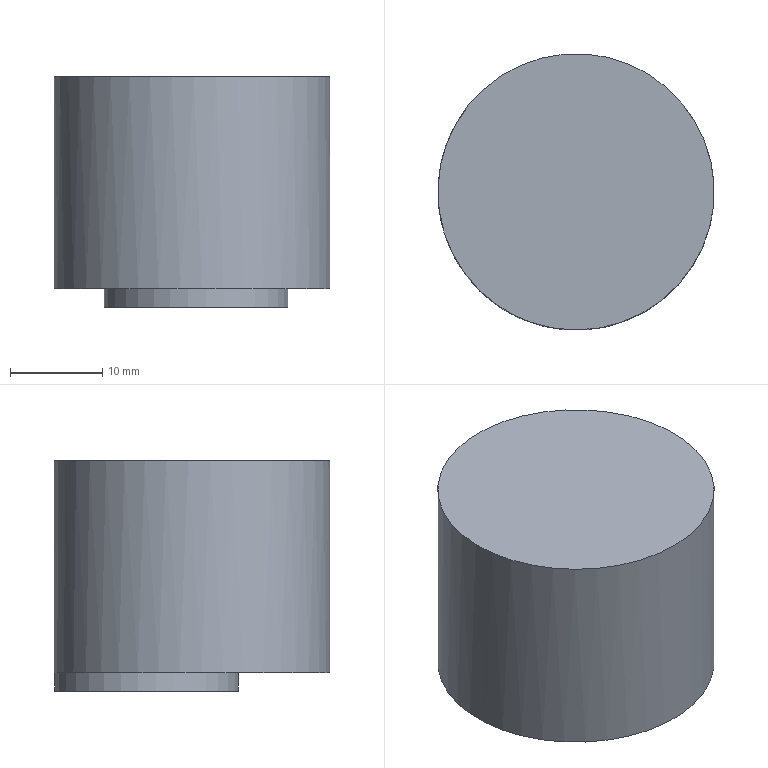Part | STEP file | gslz 2016.10.28-13_id506_x_t | 1 solid | 5 faces | box 30 x 30 x 25 mm | volume 16886 mm3 | plane 3 | cylinder 2 | commonest cylinder face diameters 20 x1 30 x1
STEP:
#1=CARTESIAN_POINT('',(0.,0.,0.));
#2=DIRECTION('',(0.,0.,1.));
#3=DIRECTION('',(1.,0.,0.));
#4=AXIS2_PLACEMENT_3D('',#1,#2,#3);
#5=CARTESIAN_POINT('',(-1110.004,-65.108,-3.75));
#6=VERTEX_POINT('',#5);
#7=CARTESIAN_POINT('',(-1087.023,-45.824,-3.75));
#8=VERTEX_POINT('',#7);
#9=CARTESIAN_POINT('',(-1098.514,-55.466,-3.75));
#10=DIRECTION('',(0.,0.,1.));
#11=DIRECTION('',(-0.766,-0.6428,0.));
#12=AXIS2_PLACEMENT_3D('',#9,#10,#11);
#13=CIRCLE('',#12,15.);
#14=CARTESIAN_POINT('',(-1051.805,-31.984,-3.75));
#15=DIRECTION('',(0.,0.,-1.));
#16=DIRECTION('',(0.1219,0.9925,0.));
#17=AXIS2_PLACEMENT_3D('',#14,#15,#16);
#18=PLANE('',#17);
#19=CARTESIAN_POINT('',(-39.971,-53.728));
#20=CARTESIAN_POINT('',(-57.689,-34.726));
#21=CARTESIAN_POINT('',(-32.374,-28.882));
#22=CARTESIAN_POINT('',(-7.059,-23.039));
#23=CARTESIAN_POINT('',(-14.656,-47.884));
#24=CARTESIAN_POINT('',(-22.252,-72.729));
#25=CARTESIAN_POINT('',(-39.971,-53.728));
#26=(BOUNDED_CURVE()B_SPLINE_CURVE(2,(#19,#20,#21,#22,#23,#24,#25),.UNSPECIFIED.,.T.,.F.)B_SPLINE_CURVE_WITH_KNOTS((1,2,2,2,2,1),(-2.094,0.,2.094,4.189,6.283,8.378),.UNSPECIFIED.)CURVE()GEOMETRIC_REPRESENTATION_ITEM()RATIONAL_B_SPLINE_CURVE((1.,0.5,1.,0.5,1.,0.5,1.))REPRESENTATION_ITEM(''));
#27=(GEOMETRIC_REPRESENTATION_CONTEXT(2)PARAMETRIC_REPRESENTATION_CONTEXT()REPRESENTATION_CONTEXT('',''));
#28=DEFINITIONAL_REPRESENTATION('',(#26),#27);
#29=PCURVE('',#18,#28);
#30=CARTESIAN_POINT('',(-1098.514,-55.466,-158.95));
#31=DIRECTION('',(0.,0.,1.));
#32=DIRECTION('',(0.766,0.6428,0.));
#33=AXIS2_PLACEMENT_3D('',#30,#31,#32);
#34=CYLINDRICAL_SURFACE('',#33,15.);
#35=CARTESIAN_POINT('',(3.142,155.2));
#36=DIRECTION('',(1.,0.));
#37=VECTOR('',#36,1.);
#38=LINE('',#35,#37);
#39=(GEOMETRIC_REPRESENTATION_CONTEXT(2)PARAMETRIC_REPRESENTATION_CONTEXT()REPRESENTATION_CONTEXT('',''));
#40=DEFINITIONAL_REPRESENTATION('',(#38),#39);
#41=PCURVE('',#34,#40);
#42=SURFACE_CURVE('',#13,(#29,#41),.PCURVE_S1.);
#43=EDGE_CURVE('',#6,#8,#42,.T.);
#44=ORIENTED_EDGE('',*,*,#43,.F.);
#45=CARTESIAN_POINT('',(-1098.514,-55.466,-3.75));
#46=DIRECTION('',(0.,0.,1.));
#47=DIRECTION('',(-0.766,-0.6428,0.));
#48=AXIS2_PLACEMENT_3D('',#45,#46,#47);
#49=CIRCLE('',#48,15.);
#50=CARTESIAN_POINT('',(-39.971,-53.728));
#51=CARTESIAN_POINT('',(-57.689,-34.726));
#52=CARTESIAN_POINT('',(-32.374,-28.882));
#53=CARTESIAN_POINT('',(-7.059,-23.039));
#54=CARTESIAN_POINT('',(-14.656,-47.884));
#55=CARTESIAN_POINT('',(-22.252,-72.729));
#56=CARTESIAN_POINT('',(-39.971,-53.728));
#57=(BOUNDED_CURVE()B_SPLINE_CURVE(2,(#50,#51,#52,#53,#54,#55,#56),.UNSPECIFIED.,.T.,.F.)B_SPLINE_CURVE_WITH_KNOTS((1,2,2,2,2,1),(-2.094,0.,2.094,4.189,6.283,8.378),.UNSPECIFIED.)CURVE()GEOMETRIC_REPRESENTATION_ITEM()RATIONAL_B_SPLINE_CURVE((1.,0.5,1.,0.5,1.,0.5,1.))REPRESENTATION_ITEM(''));
#58=(GEOMETRIC_REPRESENTATION_CONTEXT(2)PARAMETRIC_REPRESENTATION_CONTEXT()REPRESENTATION_CONTEXT('',''));
#59=DEFINITIONAL_REPRESENTATION('',(#57),#58);
#60=PCURVE('',#18,#59);
#61=CARTESIAN_POINT('',(-3.142,155.2));
#62=DIRECTION('',(1.,0.));
#63=VECTOR('',#62,1.);
#64=LINE('',#61,#63);
#65=(GEOMETRIC_REPRESENTATION_CONTEXT(2)PARAMETRIC_REPRESENTATION_CONTEXT()REPRESENTATION_CONTEXT('',''));
#66=DEFINITIONAL_REPRESENTATION('',(#64),#65);
#67=PCURVE('',#34,#66);
#68=SURFACE_CURVE('',#49,(#60,#67),.PCURVE_S1.);
#69=EDGE_CURVE('',#8,#6,#68,.T.);
#70=ORIENTED_EDGE('',*,*,#69,.F.);
#71=EDGE_LOOP('',(#44,#70));
#72=FACE_BOUND('',#71,.T.);
#73=CARTESIAN_POINT('',(-1090.422,-44.107,-3.75));
#74=VERTEX_POINT('',#73);
#75=CARTESIAN_POINT('',(-1098.082,-50.535,-3.75));
#76=DIRECTION('',(0.,0.,1.));
#77=DIRECTION('',(0.766,0.6428,0.));
#78=AXIS2_PLACEMENT_3D('',#75,#76,#77);
#79=CIRCLE('',#78,10.);
#80=CARTESIAN_POINT('',(-16.74,-36.851));
#81=CARTESIAN_POINT('',(-4.927,-49.519));
#82=CARTESIAN_POINT('',(-21.804,-53.415));
#83=CARTESIAN_POINT('',(-38.681,-57.311));
#84=CARTESIAN_POINT('',(-33.616,-40.747));
#85=CARTESIAN_POINT('',(-28.552,-24.183));
#86=CARTESIAN_POINT('',(-16.74,-36.851));
#87=(BOUNDED_CURVE()B_SPLINE_CURVE(2,(#80,#81,#82,#83,#84,#85,#86),.UNSPECIFIED.,.T.,.F.)B_SPLINE_CURVE_WITH_KNOTS((1,2,2,2,2,1),(-2.094,0.,2.094,4.189,6.283,8.378),.UNSPECIFIED.)CURVE()GEOMETRIC_REPRESENTATION_ITEM()RATIONAL_B_SPLINE_CURVE((1.,0.5,1.,0.5,1.,0.5,1.))REPRESENTATION_ITEM(''));
#88=(GEOMETRIC_REPRESENTATION_CONTEXT(2)PARAMETRIC_REPRESENTATION_CONTEXT()REPRESENTATION_CONTEXT('',''));
#89=DEFINITIONAL_REPRESENTATION('',(#87),#88);
#90=PCURVE('',#18,#89);
#91=CARTESIAN_POINT('',(-1098.082,-50.535,-5.75));
#92=DIRECTION('',(0.,0.,1.));
#93=DIRECTION('',(0.766,0.6428,0.));
#94=AXIS2_PLACEMENT_3D('',#91,#92,#93);
#95=CYLINDRICAL_SURFACE('',#94,10.);
#96=CARTESIAN_POINT('',(0.,2.));
#97=DIRECTION('',(1.,0.));
#98=VECTOR('',#97,1.);
#99=LINE('',#96,#98);
#100=(GEOMETRIC_REPRESENTATION_CONTEXT(2)PARAMETRIC_REPRESENTATION_CONTEXT()REPRESENTATION_CONTEXT('',''));
#101=DEFINITIONAL_REPRESENTATION('',(#99),#100);
#102=PCURVE('',#95,#101);
#103=SURFACE_CURVE('',#79,(#90,#102),.PCURVE_S1.);
#104=EDGE_CURVE('',#74,#74,#103,.T.);
#105=ORIENTED_EDGE('',*,*,#104,.T.);
#106=EDGE_LOOP('',(#105));
#107=FACE_BOUND('',#106,.T.);
#108=ADVANCED_FACE('',(#72,#107),#18,.T.);
#109=CARTESIAN_POINT('',(-1087.023,-45.824,19.25));
#110=VERTEX_POINT('',#109);
#111=CARTESIAN_POINT('',(-1098.514,-55.466,19.25));
#112=DIRECTION('',(0.,0.,1.));
#113=DIRECTION('',(0.766,0.6428,0.));
#114=AXIS2_PLACEMENT_3D('',#111,#112,#113);
#115=CIRCLE('',#114,15.);
#116=CARTESIAN_POINT('',(-1098.514,-55.466,19.25));
#117=DIRECTION('',(0.,0.,1.));
#118=DIRECTION('',(0.766,0.6428,0.));
#119=AXIS2_PLACEMENT_3D('',#116,#117,#118);
#120=PLANE('',#119);
#121=CARTESIAN_POINT('',(0.,0.));
#122=DIRECTION('',(1.,0.));
#123=AXIS2_PLACEMENT_2D('',#121,#122);
#124=CIRCLE('',#123,15.);
#125=(GEOMETRIC_REPRESENTATION_CONTEXT(2)PARAMETRIC_REPRESENTATION_CONTEXT()REPRESENTATION_CONTEXT('',''));
#126=DEFINITIONAL_REPRESENTATION('',(#124),#125);
#127=PCURVE('',#120,#126);
#128=CARTESIAN_POINT('',(0.,178.2));
#129=DIRECTION('',(1.,0.));
#130=VECTOR('',#129,1.);
#131=LINE('',#128,#130);
#132=(GEOMETRIC_REPRESENTATION_CONTEXT(2)PARAMETRIC_REPRESENTATION_CONTEXT()REPRESENTATION_CONTEXT('',''));
#133=DEFINITIONAL_REPRESENTATION('',(#131),#132);
#134=PCURVE('',#34,#133);
#135=SURFACE_CURVE('',#115,(#127,#134),.PCURVE_S1.);
#136=EDGE_CURVE('',#110,#110,#135,.T.);
#137=ORIENTED_EDGE('',*,*,#136,.T.);
#138=EDGE_LOOP('',(#137));
#139=FACE_BOUND('',#138,.T.);
#140=ADVANCED_FACE('',(#139),#120,.T.);
#141=ORIENTED_EDGE('',*,*,#136,.F.);
#142=CARTESIAN_POINT('',(-1087.023,-45.824,-3.75));
#143=CARTESIAN_POINT('',(-1087.023,-45.824,19.25));
#144=B_SPLINE_CURVE_WITH_KNOTS('',1,(#142,#143),.UNSPECIFIED.,.F.,.F.,(2,2),(155.2,178.2),.PIECEWISE_BEZIER_KNOTS.);
#145=CARTESIAN_POINT('',(0.,0.));
#146=DIRECTION('',(0.,1.));
#147=VECTOR('',#146,1.);
#148=LINE('',#145,#147);
#149=(GEOMETRIC_REPRESENTATION_CONTEXT(2)PARAMETRIC_REPRESENTATION_CONTEXT()REPRESENTATION_CONTEXT('',''));
#150=DEFINITIONAL_REPRESENTATION('',(#148),#149);
#151=PCURVE('',#34,#150);
#152=CARTESIAN_POINT('',(6.283,0.));
#153=DIRECTION('',(0.,1.));
#154=VECTOR('',#153,1.);
#155=LINE('',#152,#154);
#156=(GEOMETRIC_REPRESENTATION_CONTEXT(2)PARAMETRIC_REPRESENTATION_CONTEXT()REPRESENTATION_CONTEXT('',''));
#157=DEFINITIONAL_REPRESENTATION('',(#155),#156);
#158=PCURVE('',#34,#157);
#159=SEAM_CURVE('',#144,(#151,#158),.PCURVE_S1.);
#160=EDGE_CURVE('',#8,#110,#159,.T.);
#161=ORIENTED_EDGE('',*,*,#160,.F.);
#162=ORIENTED_EDGE('',*,*,#69,.T.);
#163=ORIENTED_EDGE('',*,*,#43,.T.);
#164=ORIENTED_EDGE('',*,*,#160,.T.);
#165=EDGE_LOOP('',(#141,#161,#162,#163,#164));
#166=FACE_BOUND('',#165,.T.);
#167=ADVANCED_FACE('',(#166),#34,.T.);
#168=CARTESIAN_POINT('',(-1090.422,-44.107,-5.75));
#169=VERTEX_POINT('',#168);
#170=CARTESIAN_POINT('',(-1098.082,-50.535,-5.75));
#171=DIRECTION('',(0.,0.,1.));
#172=DIRECTION('',(0.766,0.6428,0.));
#173=AXIS2_PLACEMENT_3D('',#170,#171,#172);
#174=CIRCLE('',#173,10.);
#175=CARTESIAN_POINT('',(0.,0.));
#176=DIRECTION('',(1.,0.));
#177=VECTOR('',#176,1.);
#178=LINE('',#175,#177);
#179=(GEOMETRIC_REPRESENTATION_CONTEXT(2)PARAMETRIC_REPRESENTATION_CONTEXT()REPRESENTATION_CONTEXT('',''));
#180=DEFINITIONAL_REPRESENTATION('',(#178),#179);
#181=PCURVE('',#95,#180);
#182=CARTESIAN_POINT('',(-1098.082,-50.535,-5.75));
#183=DIRECTION('',(0.,0.,1.));
#184=DIRECTION('',(0.766,0.6428,0.));
#185=AXIS2_PLACEMENT_3D('',#182,#183,#184);
#186=PLANE('',#185);
#187=CARTESIAN_POINT('',(0.,0.));
#188=DIRECTION('',(1.,0.));
#189=AXIS2_PLACEMENT_2D('',#187,#188);
#190=CIRCLE('',#189,10.);
#191=(GEOMETRIC_REPRESENTATION_CONTEXT(2)PARAMETRIC_REPRESENTATION_CONTEXT()REPRESENTATION_CONTEXT('',''));
#192=DEFINITIONAL_REPRESENTATION('',(#190),#191);
#193=PCURVE('',#186,#192);
#194=SURFACE_CURVE('',#174,(#181,#193),.PCURVE_S1.);
#195=EDGE_CURVE('',#169,#169,#194,.T.);
#196=ORIENTED_EDGE('',*,*,#195,.T.);
#197=CARTESIAN_POINT('',(-1090.422,-44.107,-5.75));
#198=CARTESIAN_POINT('',(-1090.422,-44.107,-3.75));
#199=B_SPLINE_CURVE_WITH_KNOTS('',1,(#197,#198),.UNSPECIFIED.,.F.,.F.,(2,2),(0.,2.),.PIECEWISE_BEZIER_KNOTS.);
#200=CARTESIAN_POINT('',(6.283,0.));
#201=DIRECTION('',(0.,1.));
#202=VECTOR('',#201,1.);
#203=LINE('',#200,#202);
#204=(GEOMETRIC_REPRESENTATION_CONTEXT(2)PARAMETRIC_REPRESENTATION_CONTEXT()REPRESENTATION_CONTEXT('',''));
#205=DEFINITIONAL_REPRESENTATION('',(#203),#204);
#206=PCURVE('',#95,#205);
#207=CARTESIAN_POINT('',(0.,0.));
#208=DIRECTION('',(0.,1.));
#209=VECTOR('',#208,1.);
#210=LINE('',#207,#209);
#211=(GEOMETRIC_REPRESENTATION_CONTEXT(2)PARAMETRIC_REPRESENTATION_CONTEXT()REPRESENTATION_CONTEXT('',''));
#212=DEFINITIONAL_REPRESENTATION('',(#210),#211);
#213=PCURVE('',#95,#212);
#214=SEAM_CURVE('',#199,(#206,#213),.PCURVE_S1.);
#215=EDGE_CURVE('',#169,#74,#214,.T.);
#216=ORIENTED_EDGE('',*,*,#215,.T.);
#217=ORIENTED_EDGE('',*,*,#104,.F.);
#218=ORIENTED_EDGE('',*,*,#215,.F.);
#219=EDGE_LOOP('',(#196,#216,#217,#218));
#220=FACE_BOUND('',#219,.T.);
#221=ADVANCED_FACE('',(#220),#95,.T.);
#222=ORIENTED_EDGE('',*,*,#195,.F.);
#223=EDGE_LOOP('',(#222));
#224=FACE_BOUND('',#223,.T.);
#225=ADVANCED_FACE('',(#224),#186,.F.);
#226=CLOSED_SHELL('',(#108,#140,#167,#221,#225));
#227=MANIFOLD_SOLID_BREP('',#226);
#228=(LENGTH_UNIT()NAMED_UNIT(*)SI_UNIT(.MILLI.,.METRE.));
#229=UNCERTAINTY_MEASURE_WITH_UNIT(LENGTH_MEASURE(0.000005),#228,'','');
#230=(NAMED_UNIT(*)PLANE_ANGLE_UNIT()SI_UNIT($,.RADIAN.));
#231=(NAMED_UNIT(*)SI_UNIT($,.STERADIAN.)SOLID_ANGLE_UNIT());
#232=(GEOMETRIC_REPRESENTATION_CONTEXT(3)GLOBAL_UNCERTAINTY_ASSIGNED_CONTEXT((#229))GLOBAL_UNIT_ASSIGNED_CONTEXT((#228,#230,#231))REPRESENTATION_CONTEXT('',''));
#233=ADVANCED_BREP_SHAPE_REPRESENTATION('',(#4,#227),#232);